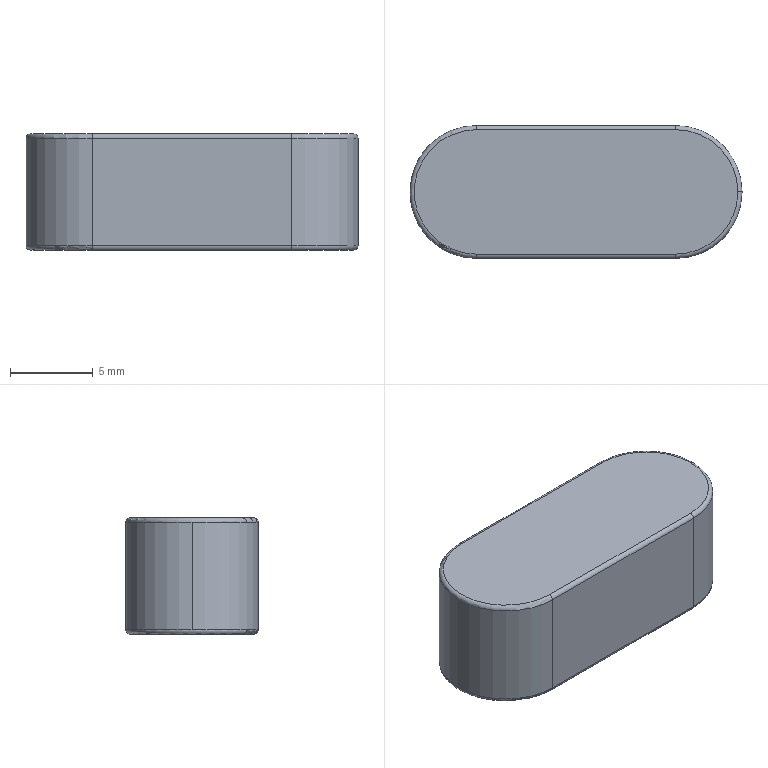Part | SolidWorks | features Extrusion 1, Fillet 1 | 1 solid | 17 faces | box 20 x 8 x 7 mm | volume 1023 mm3 | cylinder 7 | torus 6 | plane 4 | commonest cylinder face diameters 0.5 x4 8 x3
STEP:
#1=CARTESIAN_POINT('',(9.75,0.,0.));
#2=VERTEX_POINT('',#1);
#3=CARTESIAN_POINT('',(6.,-3.75,0.));
#4=VERTEX_POINT('',#3);
#5=CARTESIAN_POINT('',(6.,0.,0.));
#6=DIRECTION('',(0.,0.,-1.));
#7=DIRECTION('',(1.,0.,0.));
#8=AXIS2_PLACEMENT_3D('',#5,#6,#7);
#9=CIRCLE('',#8,3.75);
#10=EDGE_CURVE('',#2,#4,#9,.T.);
#11=ORIENTED_EDGE('',*,*,#10,.F.);
#12=CARTESIAN_POINT('',(10.,0.,0.25));
#13=VERTEX_POINT('',#12);
#14=CARTESIAN_POINT('',(9.75,0.,0.25));
#15=DIRECTION('',(0.,-1.,0.));
#16=DIRECTION('',(0.,0.,-1.));
#17=AXIS2_PLACEMENT_3D('',#14,#15,#16);
#18=CIRCLE('',#17,0.25);
#19=EDGE_CURVE('',#2,#13,#18,.T.);
#20=ORIENTED_EDGE('',*,*,#19,.T.);
#21=CARTESIAN_POINT('',(6.,-4.,0.25));
#22=VERTEX_POINT('',#21);
#23=CARTESIAN_POINT('',(6.,0.,0.25));
#24=DIRECTION('',(0.,0.,1.));
#25=DIRECTION('',(1.,0.,0.));
#26=AXIS2_PLACEMENT_3D('',#23,#24,#25);
#27=CIRCLE('',#26,4.);
#28=EDGE_CURVE('',#22,#13,#27,.T.);
#29=ORIENTED_EDGE('',*,*,#28,.F.);
#30=CARTESIAN_POINT('',(6.,-3.75,0.25));
#31=DIRECTION('',(1.,0.,0.));
#32=DIRECTION('',(0.,0.,-1.));
#33=AXIS2_PLACEMENT_3D('',#30,#31,#32);
#34=CIRCLE('',#33,0.25);
#35=EDGE_CURVE('',#22,#4,#34,.T.);
#36=ORIENTED_EDGE('',*,*,#35,.T.);
#37=EDGE_LOOP('',(#11,#20,#29,#36));
#38=FACE_OUTER_BOUND('',#37,.T.);
#39=CARTESIAN_POINT('',(6.,0.,0.25));
#40=DIRECTION('',(0.,0.,1.));
#41=DIRECTION('',(1.,0.,0.));
#42=AXIS2_PLACEMENT_3D('',#39,#40,#41);
#43=TOROIDAL_SURFACE('',#42,3.75,0.25);
#44=ADVANCED_FACE('',(#38),#43,.T.);
#45=CARTESIAN_POINT('',(10.,0.,6.75));
#46=VERTEX_POINT('',#45);
#47=CARTESIAN_POINT('',(6.,-4.,6.75));
#48=VERTEX_POINT('',#47);
#49=CARTESIAN_POINT('',(6.,0.,6.75));
#50=DIRECTION('',(0.,0.,-1.));
#51=DIRECTION('',(1.,0.,0.));
#52=AXIS2_PLACEMENT_3D('',#49,#50,#51);
#53=CIRCLE('',#52,4.);
#54=EDGE_CURVE('',#46,#48,#53,.T.);
#55=ORIENTED_EDGE('',*,*,#54,.F.);
#56=CARTESIAN_POINT('',(9.75,0.,7.));
#57=VERTEX_POINT('',#56);
#58=CARTESIAN_POINT('',(9.75,0.,6.75));
#59=DIRECTION('',(0.,-1.,0.));
#60=DIRECTION('',(0.,0.,-1.));
#61=AXIS2_PLACEMENT_3D('',#58,#59,#60);
#62=CIRCLE('',#61,0.25);
#63=EDGE_CURVE('',#46,#57,#62,.T.);
#64=ORIENTED_EDGE('',*,*,#63,.T.);
#65=CARTESIAN_POINT('',(6.,-3.75,7.));
#66=VERTEX_POINT('',#65);
#67=CARTESIAN_POINT('',(6.,0.,7.));
#68=DIRECTION('',(0.,0.,1.));
#69=DIRECTION('',(1.,0.,0.));
#70=AXIS2_PLACEMENT_3D('',#67,#68,#69);
#71=CIRCLE('',#70,3.75);
#72=EDGE_CURVE('',#66,#57,#71,.T.);
#73=ORIENTED_EDGE('',*,*,#72,.F.);
#74=CARTESIAN_POINT('',(6.,-3.75,6.75));
#75=DIRECTION('',(1.,0.,0.));
#76=DIRECTION('',(0.,0.,-1.));
#77=AXIS2_PLACEMENT_3D('',#74,#75,#76);
#78=CIRCLE('',#77,0.25);
#79=EDGE_CURVE('',#66,#48,#78,.T.);
#80=ORIENTED_EDGE('',*,*,#79,.T.);
#81=EDGE_LOOP('',(#55,#64,#73,#80));
#82=FACE_OUTER_BOUND('',#81,.T.);
#83=CARTESIAN_POINT('',(6.,0.,6.75));
#84=DIRECTION('',(0.,0.,1.));
#85=DIRECTION('',(1.,0.,0.));
#86=AXIS2_PLACEMENT_3D('',#83,#84,#85);
#87=TOROIDAL_SURFACE('',#86,3.75,0.25);
#88=ADVANCED_FACE('',(#82),#87,.T.);
#89=CARTESIAN_POINT('',(-6.,-4.,6.75));
#90=VERTEX_POINT('',#89);
#91=CARTESIAN_POINT('',(-10.,0.,6.75));
#92=VERTEX_POINT('',#91);
#93=CARTESIAN_POINT('',(-6.,0.,6.75));
#94=DIRECTION('',(0.,0.,-1.));
#95=DIRECTION('',(1.,0.,0.));
#96=AXIS2_PLACEMENT_3D('',#93,#94,#95);
#97=CIRCLE('',#96,4.);
#98=EDGE_CURVE('',#90,#92,#97,.T.);
#99=ORIENTED_EDGE('',*,*,#98,.T.);
#100=CARTESIAN_POINT('',(-10.,0.,0.25));
#101=VERTEX_POINT('',#100);
#102=CARTESIAN_POINT('',(-10.,0.,7.));
#103=DIRECTION('',(0.,0.,-1.));
#104=VECTOR('',#103,1000.);
#105=LINE('',#102,#104);
#106=EDGE_CURVE('',#92,#101,#105,.T.);
#107=ORIENTED_EDGE('',*,*,#106,.T.);
#108=CARTESIAN_POINT('',(-6.,-4.,0.25));
#109=VERTEX_POINT('',#108);
#110=CARTESIAN_POINT('',(-6.,0.,0.25));
#111=DIRECTION('',(0.,0.,1.));
#112=DIRECTION('',(1.,0.,0.));
#113=AXIS2_PLACEMENT_3D('',#110,#111,#112);
#114=CIRCLE('',#113,4.);
#115=EDGE_CURVE('',#101,#109,#114,.T.);
#116=ORIENTED_EDGE('',*,*,#115,.T.);
#117=CARTESIAN_POINT('',(-6.,-4.,7.));
#118=DIRECTION('',(0.,0.,-1.));
#119=VECTOR('',#118,1000.);
#120=LINE('',#117,#119);
#121=EDGE_CURVE('',#90,#109,#120,.T.);
#122=ORIENTED_EDGE('',*,*,#121,.F.);
#123=EDGE_LOOP('',(#99,#107,#116,#122));
#124=FACE_OUTER_BOUND('',#123,.T.);
#125=CARTESIAN_POINT('',(-6.,0.,7.));
#126=DIRECTION('',(0.,0.,-1.));
#127=DIRECTION('',(-1.,0.,0.));
#128=AXIS2_PLACEMENT_3D('',#125,#126,#127);
#129=CYLINDRICAL_SURFACE('',#128,4.);
#130=ADVANCED_FACE('',(#124),#129,.T.);
#131=ORIENTED_EDGE('',*,*,#106,.F.);
#132=CARTESIAN_POINT('',(-6.,4.,6.75));
#133=VERTEX_POINT('',#132);
#134=CARTESIAN_POINT('',(-6.,0.,6.75));
#135=DIRECTION('',(0.,0.,-1.));
#136=DIRECTION('',(1.,0.,0.));
#137=AXIS2_PLACEMENT_3D('',#134,#135,#136);
#138=CIRCLE('',#137,4.);
#139=EDGE_CURVE('',#92,#133,#138,.T.);
#140=ORIENTED_EDGE('',*,*,#139,.T.);
#141=CARTESIAN_POINT('',(-6.,4.,0.25));
#142=VERTEX_POINT('',#141);
#143=CARTESIAN_POINT('',(-6.,4.,7.));
#144=DIRECTION('',(0.,0.,-1.));
#145=VECTOR('',#144,1000.);
#146=LINE('',#143,#145);
#147=EDGE_CURVE('',#133,#142,#146,.T.);
#148=ORIENTED_EDGE('',*,*,#147,.T.);
#149=CARTESIAN_POINT('',(-6.,0.,0.25));
#150=DIRECTION('',(0.,0.,1.));
#151=DIRECTION('',(1.,0.,0.));
#152=AXIS2_PLACEMENT_3D('',#149,#150,#151);
#153=CIRCLE('',#152,4.);
#154=EDGE_CURVE('',#142,#101,#153,.T.);
#155=ORIENTED_EDGE('',*,*,#154,.T.);
#156=EDGE_LOOP('',(#131,#140,#148,#155));
#157=FACE_OUTER_BOUND('',#156,.T.);
#158=CARTESIAN_POINT('',(-6.,0.,7.));
#159=DIRECTION('',(0.,0.,-1.));
#160=DIRECTION('',(-1.,0.,0.));
#161=AXIS2_PLACEMENT_3D('',#158,#159,#160);
#162=CYLINDRICAL_SURFACE('',#161,4.);
#163=ADVANCED_FACE('',(#157),#162,.T.);
#164=CARTESIAN_POINT('',(6.,-4.,7.));
#165=DIRECTION('',(0.,0.,-1.));
#166=VECTOR('',#165,1000.);
#167=LINE('',#164,#166);
#168=EDGE_CURVE('',#48,#22,#167,.T.);
#169=ORIENTED_EDGE('',*,*,#168,.F.);
#170=CARTESIAN_POINT('',(-6.,-4.,6.75));
#171=DIRECTION('',(-1.,0.,0.));
#172=VECTOR('',#171,1000.);
#173=LINE('',#170,#172);
#174=EDGE_CURVE('',#48,#90,#173,.T.);
#175=ORIENTED_EDGE('',*,*,#174,.T.);
#176=ORIENTED_EDGE('',*,*,#121,.T.);
#177=CARTESIAN_POINT('',(-6.,-4.,0.25));
#178=DIRECTION('',(1.,0.,0.));
#179=VECTOR('',#178,1000.);
#180=LINE('',#177,#179);
#181=EDGE_CURVE('',#109,#22,#180,.T.);
#182=ORIENTED_EDGE('',*,*,#181,.T.);
#183=EDGE_LOOP('',(#169,#175,#176,#182));
#184=FACE_OUTER_BOUND('',#183,.T.);
#185=CARTESIAN_POINT('',(-6.,-4.,7.));
#186=DIRECTION('',(0.,1.,0.));
#187=DIRECTION('',(0.,0.,1.));
#188=AXIS2_PLACEMENT_3D('',#185,#186,#187);
#189=PLANE('',#188);
#190=ADVANCED_FACE('',(#184),#189,.F.);
#191=CARTESIAN_POINT('',(6.,4.,6.75));
#192=VERTEX_POINT('',#191);
#193=CARTESIAN_POINT('',(6.,4.,0.25));
#194=VERTEX_POINT('',#193);
#195=CARTESIAN_POINT('',(6.,4.,7.));
#196=DIRECTION('',(0.,0.,-1.));
#197=VECTOR('',#196,1000.);
#198=LINE('',#195,#197);
#199=EDGE_CURVE('',#192,#194,#198,.T.);
#200=ORIENTED_EDGE('',*,*,#199,.F.);
#201=CARTESIAN_POINT('',(6.,0.,6.75));
#202=DIRECTION('',(0.,0.,-1.));
#203=DIRECTION('',(1.,0.,0.));
#204=AXIS2_PLACEMENT_3D('',#201,#202,#203);
#205=CIRCLE('',#204,4.);
#206=EDGE_CURVE('',#192,#46,#205,.T.);
#207=ORIENTED_EDGE('',*,*,#206,.T.);
#208=ORIENTED_EDGE('',*,*,#54,.T.);
#209=ORIENTED_EDGE('',*,*,#168,.T.);
#210=ORIENTED_EDGE('',*,*,#28,.T.);
#211=CARTESIAN_POINT('',(6.,0.,0.25));
#212=DIRECTION('',(0.,0.,1.));
#213=DIRECTION('',(1.,0.,0.));
#214=AXIS2_PLACEMENT_3D('',#211,#212,#213);
#215=CIRCLE('',#214,4.);
#216=EDGE_CURVE('',#13,#194,#215,.T.);
#217=ORIENTED_EDGE('',*,*,#216,.T.);
#218=EDGE_LOOP('',(#200,#207,#208,#209,#210,#217));
#219=FACE_OUTER_BOUND('',#218,.T.);
#220=CARTESIAN_POINT('',(6.,0.,7.));
#221=DIRECTION('',(0.,0.,-1.));
#222=DIRECTION('',(-1.,0.,0.));
#223=AXIS2_PLACEMENT_3D('',#220,#221,#222);
#224=CYLINDRICAL_SURFACE('',#223,4.);
#225=ADVANCED_FACE('',(#219),#224,.T.);
#226=ORIENTED_EDGE('',*,*,#147,.F.);
#227=CARTESIAN_POINT('',(6.,4.,6.75));
#228=DIRECTION('',(1.,0.,0.));
#229=VECTOR('',#228,1000.);
#230=LINE('',#227,#229);
#231=EDGE_CURVE('',#133,#192,#230,.T.);
#232=ORIENTED_EDGE('',*,*,#231,.T.);
#233=ORIENTED_EDGE('',*,*,#199,.T.);
#234=CARTESIAN_POINT('',(-6.,4.,0.25));
#235=DIRECTION('',(-1.,0.,0.));
#236=VECTOR('',#235,1000.);
#237=LINE('',#234,#236);
#238=EDGE_CURVE('',#194,#142,#237,.T.);
#239=ORIENTED_EDGE('',*,*,#238,.T.);
#240=EDGE_LOOP('',(#226,#232,#233,#239));
#241=FACE_OUTER_BOUND('',#240,.T.);
#242=CARTESIAN_POINT('',(-6.,4.,7.));
#243=DIRECTION('',(0.,-1.,0.));
#244=DIRECTION('',(0.,0.,-1.));
#245=AXIS2_PLACEMENT_3D('',#242,#243,#244);
#246=PLANE('',#245);
#247=ADVANCED_FACE('',(#241),#246,.F.);
#248=CARTESIAN_POINT('',(-6.,-3.75,7.));
#249=VERTEX_POINT('',#248);
#250=CARTESIAN_POINT('',(6.,-3.75,7.));
#251=DIRECTION('',(1.,0.,0.));
#252=VECTOR('',#251,1000.);
#253=LINE('',#250,#252);
#254=EDGE_CURVE('',#249,#66,#253,.T.);
#255=ORIENTED_EDGE('',*,*,#254,.T.);
#256=ORIENTED_EDGE('',*,*,#72,.T.);
#257=CARTESIAN_POINT('',(6.,3.75,7.));
#258=VERTEX_POINT('',#257);
#259=CARTESIAN_POINT('',(6.,0.,7.));
#260=DIRECTION('',(0.,0.,1.));
#261=DIRECTION('',(1.,0.,0.));
#262=AXIS2_PLACEMENT_3D('',#259,#260,#261);
#263=CIRCLE('',#262,3.75);
#264=EDGE_CURVE('',#57,#258,#263,.T.);
#265=ORIENTED_EDGE('',*,*,#264,.T.);
#266=CARTESIAN_POINT('',(-6.,3.75,7.));
#267=VERTEX_POINT('',#266);
#268=CARTESIAN_POINT('',(-6.,3.75,7.));
#269=DIRECTION('',(-1.,0.,0.));
#270=VECTOR('',#269,1000.);
#271=LINE('',#268,#270);
#272=EDGE_CURVE('',#258,#267,#271,.T.);
#273=ORIENTED_EDGE('',*,*,#272,.T.);
#274=CARTESIAN_POINT('',(-6.,0.,7.));
#275=DIRECTION('',(0.,0.,1.));
#276=DIRECTION('',(1.,0.,0.));
#277=AXIS2_PLACEMENT_3D('',#274,#275,#276);
#278=CIRCLE('',#277,3.75);
#279=EDGE_CURVE('',#267,#249,#278,.T.);
#280=ORIENTED_EDGE('',*,*,#279,.T.);
#281=EDGE_LOOP('',(#255,#256,#265,#273,#280));
#282=FACE_OUTER_BOUND('',#281,.T.);
#283=CARTESIAN_POINT('',(-6.,0.,7.));
#284=DIRECTION('',(0.,0.,1.));
#285=DIRECTION('',(1.,0.,0.));
#286=AXIS2_PLACEMENT_3D('',#283,#284,#285);
#287=PLANE('',#286);
#288=ADVANCED_FACE('',(#282),#287,.T.);
#289=CARTESIAN_POINT('',(-6.,3.75,0.));
#290=VERTEX_POINT('',#289);
#291=CARTESIAN_POINT('',(6.,3.75,0.));
#292=VERTEX_POINT('',#291);
#293=CARTESIAN_POINT('',(-6.,3.75,0.));
#294=DIRECTION('',(1.,0.,0.));
#295=VECTOR('',#294,1000.);
#296=LINE('',#293,#295);
#297=EDGE_CURVE('',#290,#292,#296,.T.);
#298=ORIENTED_EDGE('',*,*,#297,.T.);
#299=CARTESIAN_POINT('',(6.,0.,0.));
#300=DIRECTION('',(0.,0.,-1.));
#301=DIRECTION('',(1.,0.,0.));
#302=AXIS2_PLACEMENT_3D('',#299,#300,#301);
#303=CIRCLE('',#302,3.75);
#304=EDGE_CURVE('',#292,#2,#303,.T.);
#305=ORIENTED_EDGE('',*,*,#304,.T.);
#306=ORIENTED_EDGE('',*,*,#10,.T.);
#307=CARTESIAN_POINT('',(-6.,-3.75,0.));
#308=VERTEX_POINT('',#307);
#309=CARTESIAN_POINT('',(-6.,-3.75,0.));
#310=DIRECTION('',(-1.,0.,0.));
#311=VECTOR('',#310,1000.);
#312=LINE('',#309,#311);
#313=EDGE_CURVE('',#4,#308,#312,.T.);
#314=ORIENTED_EDGE('',*,*,#313,.T.);
#315=CARTESIAN_POINT('',(-6.,0.,0.));
#316=DIRECTION('',(0.,0.,-1.));
#317=DIRECTION('',(1.,0.,0.));
#318=AXIS2_PLACEMENT_3D('',#315,#316,#317);
#319=CIRCLE('',#318,3.75);
#320=EDGE_CURVE('',#308,#290,#319,.T.);
#321=ORIENTED_EDGE('',*,*,#320,.T.);
#322=EDGE_LOOP('',(#298,#305,#306,#314,#321));
#323=FACE_OUTER_BOUND('',#322,.T.);
#324=CARTESIAN_POINT('',(-6.,0.,0.));
#325=DIRECTION('',(0.,0.,1.));
#326=DIRECTION('',(1.,0.,0.));
#327=AXIS2_PLACEMENT_3D('',#324,#325,#326);
#328=PLANE('',#327);
#329=ADVANCED_FACE('',(#323),#328,.F.);
#330=CARTESIAN_POINT('',(-6.,3.75,6.75));
#331=DIRECTION('',(1.,0.,0.));
#332=DIRECTION('',(0.,0.,-1.));
#333=AXIS2_PLACEMENT_3D('',#330,#331,#332);
#334=CIRCLE('',#333,0.25);
#335=EDGE_CURVE('',#133,#267,#334,.T.);
#336=ORIENTED_EDGE('',*,*,#335,.F.);
#337=ORIENTED_EDGE('',*,*,#139,.F.);
#338=ORIENTED_EDGE('',*,*,#98,.F.);
#339=CARTESIAN_POINT('',(-6.,-3.75,6.75));
#340=DIRECTION('',(1.,0.,0.));
#341=DIRECTION('',(0.,0.,-1.));
#342=AXIS2_PLACEMENT_3D('',#339,#340,#341);
#343=CIRCLE('',#342,0.25);
#344=EDGE_CURVE('',#249,#90,#343,.T.);
#345=ORIENTED_EDGE('',*,*,#344,.F.);
#346=ORIENTED_EDGE('',*,*,#279,.F.);
#347=EDGE_LOOP('',(#336,#337,#338,#345,#346));
#348=FACE_OUTER_BOUND('',#347,.T.);
#349=CARTESIAN_POINT('',(-6.,0.,6.75));
#350=DIRECTION('',(0.,0.,1.));
#351=DIRECTION('',(1.,0.,0.));
#352=AXIS2_PLACEMENT_3D('',#349,#350,#351);
#353=TOROIDAL_SURFACE('',#352,3.75,0.25);
#354=ADVANCED_FACE('',(#348),#353,.T.);
#355=ORIENTED_EDGE('',*,*,#344,.T.);
#356=ORIENTED_EDGE('',*,*,#174,.F.);
#357=ORIENTED_EDGE('',*,*,#79,.F.);
#358=ORIENTED_EDGE('',*,*,#254,.F.);
#359=EDGE_LOOP('',(#355,#356,#357,#358));
#360=FACE_OUTER_BOUND('',#359,.T.);
#361=CARTESIAN_POINT('',(-6.,-3.75,6.75));
#362=DIRECTION('',(-1.,0.,0.));
#363=DIRECTION('',(0.,0.,1.));
#364=AXIS2_PLACEMENT_3D('',#361,#362,#363);
#365=CYLINDRICAL_SURFACE('',#364,0.25);
#366=ADVANCED_FACE('',(#360),#365,.T.);
#367=ORIENTED_EDGE('',*,*,#335,.T.);
#368=ORIENTED_EDGE('',*,*,#272,.F.);
#369=CARTESIAN_POINT('',(6.,3.75,6.75));
#370=DIRECTION('',(1.,0.,0.));
#371=DIRECTION('',(0.,0.,-1.));
#372=AXIS2_PLACEMENT_3D('',#369,#370,#371);
#373=CIRCLE('',#372,0.25);
#374=EDGE_CURVE('',#192,#258,#373,.T.);
#375=ORIENTED_EDGE('',*,*,#374,.F.);
#376=ORIENTED_EDGE('',*,*,#231,.F.);
#377=EDGE_LOOP('',(#367,#368,#375,#376));
#378=FACE_OUTER_BOUND('',#377,.T.);
#379=CARTESIAN_POINT('',(-6.,3.75,6.75));
#380=DIRECTION('',(1.,0.,0.));
#381=DIRECTION('',(0.,0.,-1.));
#382=AXIS2_PLACEMENT_3D('',#379,#380,#381);
#383=CYLINDRICAL_SURFACE('',#382,0.25);
#384=ADVANCED_FACE('',(#378),#383,.T.);
#385=ORIENTED_EDGE('',*,*,#63,.F.);
#386=ORIENTED_EDGE('',*,*,#206,.F.);
#387=ORIENTED_EDGE('',*,*,#374,.T.);
#388=ORIENTED_EDGE('',*,*,#264,.F.);
#389=EDGE_LOOP('',(#385,#386,#387,#388));
#390=FACE_OUTER_BOUND('',#389,.T.);
#391=CARTESIAN_POINT('',(6.,0.,6.75));
#392=DIRECTION('',(0.,0.,1.));
#393=DIRECTION('',(1.,0.,0.));
#394=AXIS2_PLACEMENT_3D('',#391,#392,#393);
#395=TOROIDAL_SURFACE('',#394,3.75,0.25);
#396=ADVANCED_FACE('',(#390),#395,.T.);
#397=CARTESIAN_POINT('',(-6.,3.75,0.25));
#398=DIRECTION('',(1.,0.,0.));
#399=DIRECTION('',(0.,0.,-1.));
#400=AXIS2_PLACEMENT_3D('',#397,#398,#399);
#401=CIRCLE('',#400,0.25);
#402=EDGE_CURVE('',#290,#142,#401,.T.);
#403=ORIENTED_EDGE('',*,*,#402,.F.);
#404=ORIENTED_EDGE('',*,*,#320,.F.);
#405=CARTESIAN_POINT('',(-6.,-3.75,0.25));
#406=DIRECTION('',(1.,0.,0.));
#407=DIRECTION('',(0.,0.,-1.));
#408=AXIS2_PLACEMENT_3D('',#405,#406,#407);
#409=CIRCLE('',#408,0.25);
#410=EDGE_CURVE('',#109,#308,#409,.T.);
#411=ORIENTED_EDGE('',*,*,#410,.F.);
#412=ORIENTED_EDGE('',*,*,#115,.F.);
#413=ORIENTED_EDGE('',*,*,#154,.F.);
#414=EDGE_LOOP('',(#403,#404,#411,#412,#413));
#415=FACE_OUTER_BOUND('',#414,.T.);
#416=CARTESIAN_POINT('',(-6.,0.,0.25));
#417=DIRECTION('',(0.,0.,1.));
#418=DIRECTION('',(1.,0.,0.));
#419=AXIS2_PLACEMENT_3D('',#416,#417,#418);
#420=TOROIDAL_SURFACE('',#419,3.75,0.25);
#421=ADVANCED_FACE('',(#415),#420,.T.);
#422=ORIENTED_EDGE('',*,*,#410,.T.);
#423=ORIENTED_EDGE('',*,*,#313,.F.);
#424=ORIENTED_EDGE('',*,*,#35,.F.);
#425=ORIENTED_EDGE('',*,*,#181,.F.);
#426=EDGE_LOOP('',(#422,#423,#424,#425));
#427=FACE_OUTER_BOUND('',#426,.T.);
#428=CARTESIAN_POINT('',(-6.,-3.75,0.25));
#429=DIRECTION('',(1.,0.,0.));
#430=DIRECTION('',(0.,0.,-1.));
#431=AXIS2_PLACEMENT_3D('',#428,#429,#430);
#432=CYLINDRICAL_SURFACE('',#431,0.25);
#433=ADVANCED_FACE('',(#427),#432,.T.);
#434=ORIENTED_EDGE('',*,*,#402,.T.);
#435=ORIENTED_EDGE('',*,*,#238,.F.);
#436=CARTESIAN_POINT('',(6.,3.75,0.25));
#437=DIRECTION('',(1.,0.,0.));
#438=DIRECTION('',(0.,0.,-1.));
#439=AXIS2_PLACEMENT_3D('',#436,#437,#438);
#440=CIRCLE('',#439,0.25);
#441=EDGE_CURVE('',#292,#194,#440,.T.);
#442=ORIENTED_EDGE('',*,*,#441,.F.);
#443=ORIENTED_EDGE('',*,*,#297,.F.);
#444=EDGE_LOOP('',(#434,#435,#442,#443));
#445=FACE_OUTER_BOUND('',#444,.T.);
#446=CARTESIAN_POINT('',(-6.,3.75,0.25));
#447=DIRECTION('',(-1.,0.,0.));
#448=DIRECTION('',(0.,0.,1.));
#449=AXIS2_PLACEMENT_3D('',#446,#447,#448);
#450=CYLINDRICAL_SURFACE('',#449,0.25);
#451=ADVANCED_FACE('',(#445),#450,.T.);
#452=ORIENTED_EDGE('',*,*,#19,.F.);
#453=ORIENTED_EDGE('',*,*,#304,.F.);
#454=ORIENTED_EDGE('',*,*,#441,.T.);
#455=ORIENTED_EDGE('',*,*,#216,.F.);
#456=EDGE_LOOP('',(#452,#453,#454,#455));
#457=FACE_OUTER_BOUND('',#456,.T.);
#458=CARTESIAN_POINT('',(6.,0.,0.25));
#459=DIRECTION('',(0.,0.,1.));
#460=DIRECTION('',(1.,0.,0.));
#461=AXIS2_PLACEMENT_3D('',#458,#459,#460);
#462=TOROIDAL_SURFACE('',#461,3.75,0.25);
#463=ADVANCED_FACE('',(#457),#462,.T.);
#464=CLOSED_SHELL('',(#44,#88,#130,#163,#190,#225,#247,#288,#329,#354,#366,#384,#396,#421,#433,#451,#463));
#465=MANIFOLD_SOLID_BREP('',#464);
#466=CARTESIAN_POINT('',(0.,0.,0.));
#467=DIRECTION('',(0.,0.,1.));
#468=DIRECTION('',(1.,0.,0.));
#469=AXIS2_PLACEMENT_3D('',#466,#467,#468);
#470=(LENGTH_UNIT()NAMED_UNIT(*)SI_UNIT(.MILLI.,.METRE.));
#471=UNCERTAINTY_MEASURE_WITH_UNIT(LENGTH_MEASURE(0.00001),#470,'','');
#472=(NAMED_UNIT(*)PLANE_ANGLE_UNIT()SI_UNIT($,.RADIAN.));
#473=(NAMED_UNIT(*)SI_UNIT($,.STERADIAN.)SOLID_ANGLE_UNIT());
#474=(GEOMETRIC_REPRESENTATION_CONTEXT(3)GLOBAL_UNCERTAINTY_ASSIGNED_CONTEXT((#471))GLOBAL_UNIT_ASSIGNED_CONTEXT((#470,#472,#473))REPRESENTATION_CONTEXT('',''));
#475=ADVANCED_BREP_SHAPE_REPRESENTATION('',(#465,#469),#474);